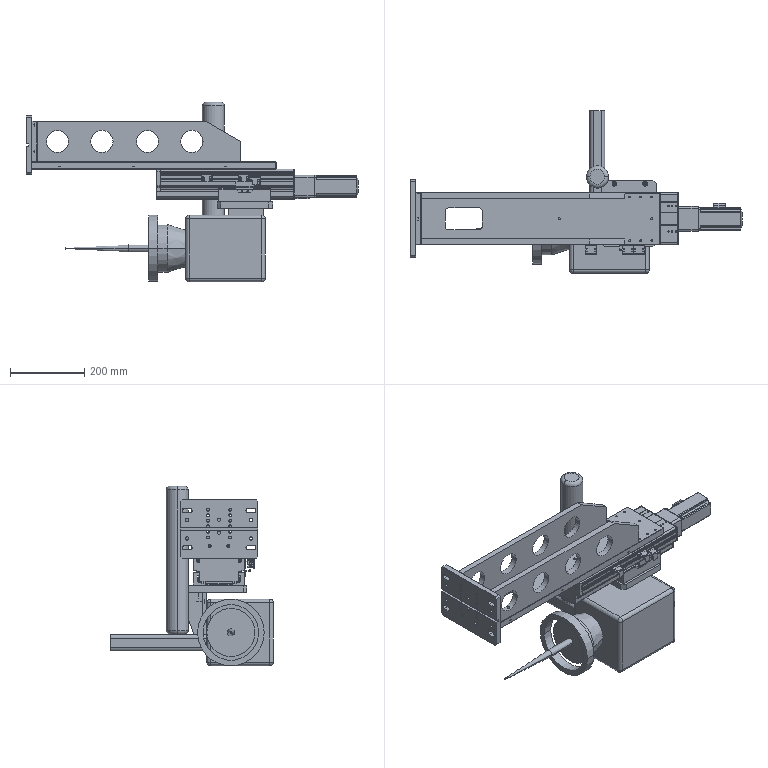Part | SolidWorks | features InContextFeatHolder 20, ReferencePattern 8, DerivedHolePattern 2, Attribute 1, MirrorCompFeat 1 | 49 solids | 2510 faces | box 896.5 x 440 x 485 mm | volume 17056339 mm3 | cylinder 1131 | plane 971 | cone 336 | torus 64 | sphere 8 | commonest cylinder face diameters 8 x150 5 x100 3.3 x76 4.5 x76 6 x58 11 x56